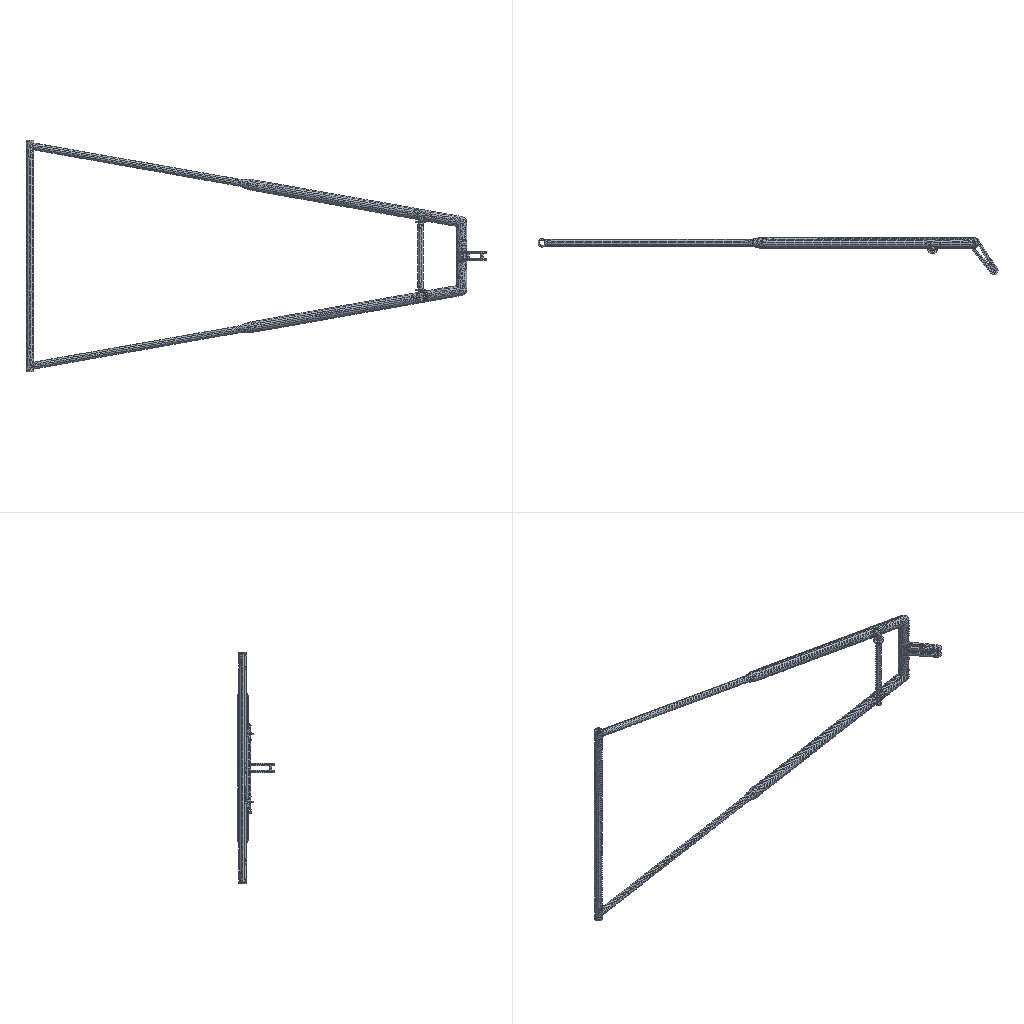Simulation study | ansys workbench
Set-up summary:
category,name,step,type,value,unit,region
solver,ansys_workbench
units,mm-N-s-tonne (MPa),,stated,"/units,MPA"
analysis,LS1,,static
load_step,LS1,LS1,static,nsubst=1; time=1
mesh,nodes,,,92059
mesh,elements,,,55127
element_type,SOLID187,,,53612
element_type,SURF154,,,1515
material,"Aluminum Alloy , Wrought , 6061 , T6",,E,69040,tonne s^-2 mm^-1
material,"Aluminum Alloy , Wrought , 6061 , T6",,nu,0.33
material,"Aluminum Alloy , Wrought , 6061 , T6",,density,2.713e-09,tonne mm^-3
material,"Aluminum Alloy , Wrought , 6061 , T6",,conductivity,155.3,tonne mm s^-3 C^-1
material,"Aluminum Alloy , Wrought , 6061 , T6",,specific_heat,9.157e+08,mm^2 s^-2 C^-1
material,"Aluminum Alloy , Wrought , 6061 , T6",,cte,2.278e-05,C^-1
load,Define Force Using Surface Effect Elements,LS1,surface-effect pres face 2,-0.01445,,SURF154 #2
load,Define Force Using Surface Effect Elements,LS1,surface-effect pres face 1,0.001275,,SURF154 #3
load,ACEL,LS1,gravity (ACEL; gravity acts opposite),"9806.65 [dir=(0, -1, 0)]",,all
bc,Fixed Supports,model,fixed,[dofs=ALL],,_FIXEDSU
named_set,_FIXEDSU,,node,5678
Ansys APDL input file, long lists of numbers shortened:
/batch
/config,noeldb,1     ! force off writing results to database
*get,_wallstrt,active,,time,wall
! ANSYS input file written by Workbench version 2021 R1
! File used for geometry attach:
/title,______--____ (B5)
! ****** Begin Custom Load Command Snippet ******
/COM, ACT Extensions:
/COM,     LSDYNA, 2021.1
/COM,
! ****** End   Custom Load Command Snippet ******
*DIM,_wb_ProjectScratch_dir,string,248
_wb_ProjectScratch_dir(1) = ''
*DIM,_wb_SolverFiles_dir,string,248
_wb_SolverFiles_dir(1) = ''
*DIM,_wb_userfiles_dir,string,248
_wb_userfiles_dir(1) = ''
/com,--- Data in consistent NMM units. See Solving Units in the help system for more information.
/units,MPA
/nopr
/wb,file,start              !  signify a WB generated input file
/prep7
! Turn off shape checking because checks already performed inside WB mesher.
! See help system for more information.
SHPP,OFF,,NOWARN
/nolist
etcon,set             ! allow ANSYS to choose best KEYOP's for 180x elements, resets any applicable keyopt to MAPDL defaults
/com,*********** Nodes for the whole assembly ***********
nblock,3,,101264
(1i9,3e20.9e3)
        1     1.738287455E+03    -2.350226247E+01     3.625000000E+02
! (92058 more lines like these left out)
-1
/wb,elem,start            !  set before creation of elements
/com,*********** Elements for Body 1 "skj3(1)-FreeParts|__-__3" ***********
et,1,187
eblock,19,solid,,53612
(19i9)
        1        1        1        1        0        0        0        0       10        0        1    13475    14341    13639    14333    90244    90732    90239    90242
! (107223 more lines like these left out)
-1
/wb,elem,end               !  done creating elements
/com,*********** Send User Defined Coordinate System(s) ***********
csys,0
toffst,273.15,  ! Temperature offset from absolute zero
/com,*********** Set Reference Temperature ***********
tref,22.
/wb,mat,start              !  starting to send materials
/com,*********** Send Materials ***********
Temperature = 'TEMP' ! Temperature
MP,DENS,1,2.713e-09,	! tonne mm^-3
MP,EX,1,69040,	! tonne s^-2 mm^-1
MP,NUXY,1,0.33,
MP,ALPX,1,2.278e-05,	! C^-1
MP,KXX,1,155.3,	! tonne mm s^-3 C^-1
MP,C,1,915700000,	! mm^2 s^-2 C^-1
/wb,mat,end                !  done sending materials
!************************* Model Summary ********************
!skj3(1)-FreeParts|__-__3,	铝合金，锻造，6061，T6,	matid,	1
!************************* End Model Summary ********************
! get the diagonal of the bounding box. Needed later for other things
*get,_xmin,node,,mnloc,x
*get,_ymin,node,,mnloc,y
*get,_zmin,node,,mnloc,z
*get,_xmax,node,,mxloc,x
*get,_ymax,node,,mxloc,y
*get,_zmax,node,,mxloc,z
_ASMDIAG=(_xmax-_xmin)*(_xmax-_xmin)+(_ymax-_ymin)*(_ymax-_ymin)+(_zmax-_zmin)*(_zmax-_zmin)
_ASMDIAG=SQRT(_ASMDIAG)
/wb,contact,start          !  starting to send contact
/wb,contact,end            !  done creating contacts
/golist
/wb,load,start             !  starting to send loads
/com,*********** Fixed Supports ***********
CMBLOCK,_FIXEDSU,NODE,     5678
(8i10)
       107       108       109       110       111       112       113       114
! (709 more lines like these left out)
cmsel,s,_FIXEDSU
d,all,all
nsel,all
/com,*********** Define Force Using Surface Effect Elements ***********
local,12,0,0.,0.,0.,0.,0.,0.
csys,0
et,2,154
eblock,10,,,530
(15i9)
    73133        2        2        2       12     1156     1155     3778     3778    23246    23248     3778    23257
! (529 more lines like these left out)
-1
esel,s,type,,2
keyop,2,2,1                ! Apply load in local coordinate system
keyop,2,7,1                ! Use original area so load is constant in large deformation
esel,all
*DIM,_loadvari30y,TABLE,2,1,1,TIME,
! Time values
_loadvari30y(1,0,1) = 0.
_loadvari30y(2,0,1) = 1.
! Load values
_loadvari30y(1,1,1) = -1.44504999276924e-002
_loadvari30y(2,1,1) = -1.44504999276924e-002
/com,*********** Define Force Using Surface Effect Elements ***********
local,13,0,0.,0.,0.,0.,0.,0.
csys,0
et,3,154
eblock,10,,,985
(15i9)
    73663        3        3        3       13     1156     1155     3778     3778    23246    23248     3778    23257
! (984 more lines like these left out)
-1
esel,s,type,,3
keyop,3,2,1                ! Apply load in local coordinate system
keyop,3,7,1                ! Use original area so load is constant in large deformation
esel,all
*DIM,_loadvari66x,TABLE,2,1,1,TIME,
! Time values
_loadvari66x(1,0,1) = 0.
_loadvari66x(2,0,1) = 1.
! Load values
_loadvari66x(1,1,1) = 1.27504988287494e-003
_loadvari66x(2,1,1) = 1.27504988287494e-003
/gst,on,on
fini
*get,_numnode,node,0,count
*get,_numelem,elem,0,count
*get, _MAXELEMNUM, elem, 0, NUM, MAX
*get, _MAXNODENUM, node, 0, NUM, MAX
*get, _MAXELEMTYPE, etyp, 0, NUM, MAX
*get, _MAXREALCONST, real, 0, NUM, MAX
/go
/wb,load,end               !  done creating loads
/com,--- Number of total nodes = %_numnode%
/com,--- Number of contact elements = 1515
/com,--- Number of spring elements = 0
/com,--- Number of bearing elements = 0
/com,--- Number of solid elements = 53612
/com,--- Number of condensed parts = 0
/com,--- Number of total elements = %_numelem%
*get,_wallbsol,active,,time,wall
/com,****************************************************************************
/com,*************************    SOLUTION       ********************************
/com,****************************************************************************
/solu
antype,0                   ! static analysis
_thickRatio=  1     ! Ratio of thick parts in the model
eqsl,pcg,1e-8,,,,,,1
cntr,print,1               ! print out contact info and also make no initial contact an error
dmpoption,emat,no             ! Don't combine emat file for DANSYS
dmpoption,esav,no             ! Don't combine esav file for DANSYS
nldiag,cont,iter           ! print out contact info each equilibrium iteration
rescontrol,,none                 ! Do not keep any restart files
/com,****************************************************
/com,******************* SOLVE FOR LS 1 OF 1 ****************
esel,s,type,,2
nsle
sfe,all,1,pres,1,0.
sfe,all,2,pres,1,%_loadvari30y%
sfe,all,3,pres,1,0.
esel,s,type,,3
nsle
sfe,all,1,pres,1,%_loadvari66x%
sfe,all,2,pres,1,0.
sfe,all,3,pres,1,0.
nsel,all
esel,all
acel,0.,9806.65,0.
/nopr
/gopr
/nolist
nsub,1,1,1
time,1.
outres,erase
outres,all,none
outres,nsol,all,
outres,rsol,all
outres,eangl,all
outres,etmp,all
outres,veng,all
outres,strs,all,
outres,epel,all,
outres,eppl,all,
outres,cont,all,
! *********** WB SOLVE COMMAND ***********
! check interactive state
*get,ANSINTER_,active,,int
*if,ANSINTER_,ne,0,then
/eof
*endif
solve
/com *************** Write FE CONNECTORS *********
CEWRITE,file,ce,,INTE
/com,****************************************************
/com,*************** FINISHED SOLVE FOR LS 1 *************
*get,_wallasol,active,,time,wall
/nopr
*get,_numnode,node,0,count
*get,_numelem,elem,0,count
*get, _MAXELEMNUM, elem, 0, NUM, MAX
*get, _MAXNODENUM, node, 0, NUM, MAX,,,INTERNAL
*get, _MAXELEMTYPE, etyp, 0, NUM, MAX
*get, _MAXREALCONST, real, 0, NUM, MAX
/gopr
*get,_PCGITER,active,,solu,cgiter
/post1
xmlo,ENCODING,ISO-8859-1
xmlo,parm
/xml,parm,xml
fini
/gopr
*get,_walldone,active,,time,wall
_preptime=(_wallbsol-_wallstrt)*3600
_solvtime=(_wallasol-_wallbsol)*3600
_posttime=(_walldone-_wallasol)*3600
_totaltim=(_walldone-_wallstrt)*3600
*get,_dlbratio,active,0,solu,dlbr
*get,_combtime,active,0,solu,comb
/com,--- Total number of nodes = %_numnode%
/com,--- Total number of elements = %_numelem%
/com,--- Element load balance ratio = %_dlbratio%
/com,--- Time to combine distributed files = %_combtime%
/wb,file,end               ! done with WB generated input
Results summary:
result,analyses[0].index,,,1
result,analyses[0].system,,,SYS-1
result,analyses[0].deck,,,deck.dat
result,analyses[0].solve_status,,,completed
result,analyses[0].analysis_type,,,static
result,analyses[0].physics,,,mechanical
result,analyses[0].unit_system,,,"NMM: mm, ton, N, s, mV, mA, degC"
result,analyses[0].n_sets,,,1
result,analyses[0].load_steps[0].set,set=1,,1
result,analyses[0].load_steps[0].time_or_freq,set=1,,1
result,analyses[0].load_steps[0].max_displacement_magnitude,set=1,,153.887
result,analyses[0].load_steps[0].max_von_mises_nodal,set=1,,141.083
result,analyses[0].load_steps[0].reaction_force_sum_xyz[1],set=1,,-49.999
result,analyses[0].load_steps[0].reaction_force_sum_xyz[2],set=1,,458.932
result,analyses[0].load_steps[0].reaction_force_sum_xyz[3],set=1,,-1.63086e-05
result,geometry_export[0][0],,,.step
result,geometry_export[0][1],,,ok
result,geometry_export[0][2],,,1